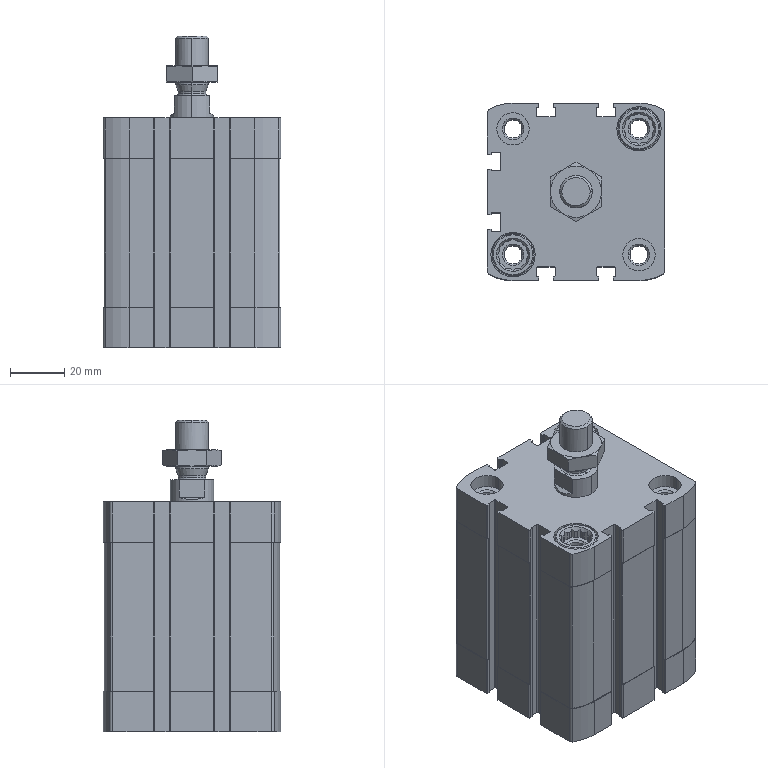Part | SolidWorks | 3 solids | 491 faces | box 65.5 x 65.5 x 115.2 mm | volume 259589 mm3 | plane 227 | cylinder 212 | cone 48 | spline 4 | commonest cylinder face diameters 0.8 x48 10.6 x48 0.4 x24 6.647 x16 12 x12 2.7 x8